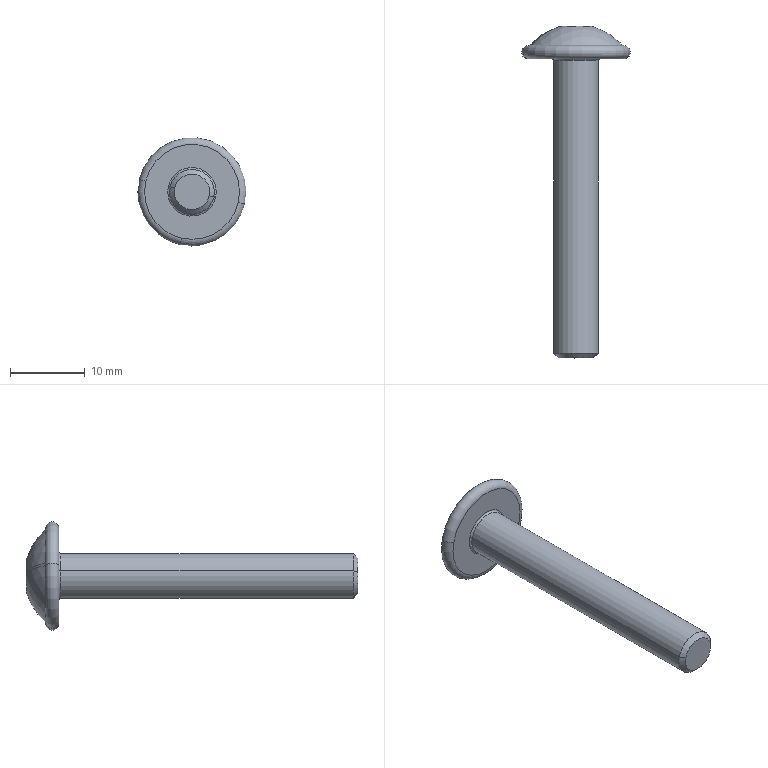Part | SolidWorks | features BaseBody 1 | 1 solid | 33 faces | box 14.5 x 44.401 x 14.5 mm | volume 1558 mm3 | cylinder 18 | torus 5 | sphere 4 | plane 4 | cone 2 | commonest cylinder face diameters 1.32 x6 3.14 x4 2.34 x3 6 x3 1.26 x2
STEP:
#1=CARTESIAN_POINT('',(2000.565,170.805,805.124));
#2=VERTEX_POINT('',#1);
#3=CARTESIAN_POINT('',(2002.818,170.805,801.529));
#4=VERTEX_POINT('',#3);
#5=CARTESIAN_POINT('',(2003.489,170.805,804.453));
#6=DIRECTION('',(0.,-1.,0.));
#7=DIRECTION('',(-0.9746,0.,0.2239));
#8=AXIS2_PLACEMENT_3D('',#5,#6,#7);
#9=CIRCLE('',#8,3.);
#10=EDGE_CURVE('',#2,#4,#9,.T.);
#11=ORIENTED_EDGE('',*,*,#10,.T.);
#12=CARTESIAN_POINT('',(2002.818,131.68,801.529));
#13=VERTEX_POINT('',#12);
#14=CARTESIAN_POINT('',(2002.818,171.588,801.529));
#15=DIRECTION('',(0.,-1.,0.));
#16=VECTOR('',#15,1000.);
#17=LINE('',#14,#16);
#18=EDGE_CURVE('',#4,#13,#17,.T.);
#19=ORIENTED_EDGE('',*,*,#18,.T.);
#20=CARTESIAN_POINT('',(2000.565,131.68,805.124));
#21=VERTEX_POINT('',#20);
#22=CARTESIAN_POINT('',(2003.489,131.68,804.453));
#23=DIRECTION('',(0.,-1.,0.));
#24=DIRECTION('',(-0.9746,0.,0.2239));
#25=AXIS2_PLACEMENT_3D('',#22,#23,#24);
#26=CIRCLE('',#25,3.);
#27=EDGE_CURVE('',#21,#13,#26,.T.);
#28=ORIENTED_EDGE('',*,*,#27,.F.);
#29=CARTESIAN_POINT('',(2000.565,170.805,805.124));
#30=DIRECTION('',(0.,-1.,0.));
#31=VECTOR('',#30,1000.);
#32=LINE('',#29,#31);
#33=EDGE_CURVE('',#2,#21,#32,.T.);
#34=ORIENTED_EDGE('',*,*,#33,.F.);
#35=EDGE_LOOP('',(#11,#19,#28,#34));
#36=FACE_OUTER_BOUND('',#35,.T.);
#37=CARTESIAN_POINT('',(2003.489,171.588,804.453));
#38=DIRECTION('',(0.,-1.,0.));
#39=DIRECTION('',(-0.2239,0.,-0.9746));
#40=AXIS2_PLACEMENT_3D('',#37,#38,#39);
#41=CYLINDRICAL_SURFACE('',#40,3.);
#42=ADVANCED_FACE('',(#36),#41,.T.);
#43=CARTESIAN_POINT('',(2003.924,175.456,806.344));
#44=VERTEX_POINT('',#43);
#45=CARTESIAN_POINT('',(2003.428,175.404,806.592));
#46=VERTEX_POINT('',#45);
#47=CARTESIAN_POINT('',(2003.924,175.456,806.344));
#48=CARTESIAN_POINT('',(2003.833,175.456,806.365));
#49=CARTESIAN_POINT('',(2003.743,175.451,806.397));
#50=CARTESIAN_POINT('',(2003.576,175.434,806.481));
#51=CARTESIAN_POINT('',(2003.499,175.421,806.532));
#52=CARTESIAN_POINT('',(2003.428,175.404,806.592));
#53=B_SPLINE_CURVE_WITH_KNOTS('',3,(#47,#48,#49,#50,#51,#52),.UNSPECIFIED.,.F.,.F.,(4,2,4),(0.0005602,0.0008404,0.001121),.UNSPECIFIED.);
#54=EDGE_CURVE('',#44,#46,#53,.T.);
#55=ORIENTED_EDGE('',*,*,#54,.F.);
#56=CARTESIAN_POINT('',(2003.924,173.205,806.344));
#57=VERTEX_POINT('',#56);
#58=CARTESIAN_POINT('',(2003.924,175.576,806.344));
#59=DIRECTION('',(0.,-1.,0.));
#60=VECTOR('',#59,1000.);
#61=LINE('',#58,#60);
#62=EDGE_CURVE('',#44,#57,#61,.T.);
#63=ORIENTED_EDGE('',*,*,#62,.T.);
#64=CARTESIAN_POINT('',(2003.428,173.205,806.592));
#65=VERTEX_POINT('',#64);
#66=CARTESIAN_POINT('',(2004.186,173.205,807.484));
#67=DIRECTION('',(0.,-1.,0.));
#68=DIRECTION('',(-0.6474,0.,-0.7622));
#69=AXIS2_PLACEMENT_3D('',#66,#67,#68);
#70=CIRCLE('',#69,1.17);
#71=EDGE_CURVE('',#65,#57,#70,.T.);
#72=ORIENTED_EDGE('',*,*,#71,.F.);
#73=CARTESIAN_POINT('',(2003.428,173.205,806.592));
#74=DIRECTION('',(0.,1.,0.));
#75=VECTOR('',#74,1000.);
#76=LINE('',#73,#75);
#77=EDGE_CURVE('',#65,#46,#76,.T.);
#78=ORIENTED_EDGE('',*,*,#77,.T.);
#79=EDGE_LOOP('',(#55,#63,#72,#78));
#80=FACE_OUTER_BOUND('',#79,.T.);
#81=CARTESIAN_POINT('',(2004.186,175.576,807.484));
#82=DIRECTION('',(0.,-1.,0.));
#83=DIRECTION('',(-0.2239,0.,-0.9746));
#84=AXIS2_PLACEMENT_3D('',#81,#82,#83);
#85=CYLINDRICAL_SURFACE('',#84,1.17);
#86=ADVANCED_FACE('',(#80),#85,.T.);
#87=CARTESIAN_POINT('',(2002.188,175.358,802.55));
#88=VERTEX_POINT('',#87);
#89=CARTESIAN_POINT('',(2002.501,175.404,802.555));
#90=VERTEX_POINT('',#89);
#91=CARTESIAN_POINT('',(2002.188,175.358,802.55));
#92=CARTESIAN_POINT('',(2002.291,175.369,802.527));
#93=CARTESIAN_POINT('',(2002.399,175.385,802.528));
#94=CARTESIAN_POINT('',(2002.501,175.404,802.555));
#95=B_SPLINE_CURVE_WITH_KNOTS('',3,(#91,#92,#93,#94),.UNSPECIFIED.,.F.,.F.,(4,4),(0.0009536,0.001271),.UNSPECIFIED.);
#96=EDGE_CURVE('',#88,#90,#95,.T.);
#97=ORIENTED_EDGE('',*,*,#96,.F.);
#98=CARTESIAN_POINT('',(2002.188,173.205,802.55));
#99=VERTEX_POINT('',#98);
#100=CARTESIAN_POINT('',(2002.188,175.524,802.55));
#101=DIRECTION('',(0.,-1.,0.));
#102=VECTOR('',#101,1000.);
#103=LINE('',#100,#102);
#104=EDGE_CURVE('',#88,#99,#103,.T.);
#105=ORIENTED_EDGE('',*,*,#104,.T.);
#106=CARTESIAN_POINT('',(2002.501,173.205,802.555));
#107=VERTEX_POINT('',#106);
#108=CARTESIAN_POINT('',(2002.336,173.205,803.194));
#109=DIRECTION('',(0.,1.,0.));
#110=DIRECTION('',(0.2499,0.,-0.9683));
#111=AXIS2_PLACEMENT_3D('',#108,#109,#110);
#112=CIRCLE('',#111,0.66);
#113=EDGE_CURVE('',#107,#99,#112,.T.);
#114=ORIENTED_EDGE('',*,*,#113,.F.);
#115=CARTESIAN_POINT('',(2002.501,173.205,802.555));
#116=DIRECTION('',(0.,1.,0.));
#117=VECTOR('',#116,1000.);
#118=LINE('',#115,#117);
#119=EDGE_CURVE('',#107,#90,#118,.T.);
#120=ORIENTED_EDGE('',*,*,#119,.T.);
#121=EDGE_LOOP('',(#97,#105,#114,#120));
#122=FACE_OUTER_BOUND('',#121,.T.);
#123=CARTESIAN_POINT('',(2002.336,175.524,803.194));
#124=DIRECTION('',(0.,-1.,0.));
#125=DIRECTION('',(-0.2239,0.,-0.9746));
#126=AXIS2_PLACEMENT_3D('',#123,#124,#125);
#127=CYLINDRICAL_SURFACE('',#126,0.66);
#128=ADVANCED_FACE('',(#122),#127,.F.);
#129=CARTESIAN_POINT('',(2003.83,175.358,802.173));
#130=VERTEX_POINT('',#129);
#131=CARTESIAN_POINT('',(2004.598,175.397,802.59));
#132=VERTEX_POINT('',#131);
#133=CARTESIAN_POINT('',(2003.83,175.358,802.173));
#134=CARTESIAN_POINT('',(2003.984,175.341,802.138));
#135=CARTESIAN_POINT('',(2004.154,175.335,802.161));
#136=CARTESIAN_POINT('',(2004.433,175.349,802.313));
#137=CARTESIAN_POINT('',(2004.543,175.369,802.441));
#138=CARTESIAN_POINT('',(2004.598,175.397,802.59));
#139=B_SPLINE_CURVE_WITH_KNOTS('',3,(#133,#134,#135,#136,#137,#138),.UNSPECIFIED.,.F.,.F.,(4,2,4),(0.0003176,0.0007942,0.001271),.UNSPECIFIED.);
#140=EDGE_CURVE('',#130,#132,#139,.T.);
#141=ORIENTED_EDGE('',*,*,#140,.F.);
#142=CARTESIAN_POINT('',(2003.83,173.205,802.173));
#143=VERTEX_POINT('',#142);
#144=CARTESIAN_POINT('',(2003.83,175.524,802.173));
#145=DIRECTION('',(0.,-1.,0.));
#146=VECTOR('',#145,1000.);
#147=LINE('',#144,#146);
#148=EDGE_CURVE('',#130,#143,#147,.T.);
#149=ORIENTED_EDGE('',*,*,#148,.T.);
#150=CARTESIAN_POINT('',(2004.598,173.205,802.59));
#151=VERTEX_POINT('',#150);
#152=CARTESIAN_POINT('',(2003.978,173.205,802.817));
#153=DIRECTION('',(0.,1.,0.));
#154=DIRECTION('',(0.9391,0.,-0.3438));
#155=AXIS2_PLACEMENT_3D('',#152,#153,#154);
#156=CIRCLE('',#155,0.66);
#157=EDGE_CURVE('',#151,#143,#156,.T.);
#158=ORIENTED_EDGE('',*,*,#157,.F.);
#159=CARTESIAN_POINT('',(2004.598,173.205,802.59));
#160=DIRECTION('',(0.,1.,0.));
#161=VECTOR('',#160,1000.);
#162=LINE('',#159,#161);
#163=EDGE_CURVE('',#151,#132,#162,.T.);
#164=ORIENTED_EDGE('',*,*,#163,.T.);
#165=EDGE_LOOP('',(#141,#149,#158,#164));
#166=FACE_OUTER_BOUND('',#165,.T.);
#167=CARTESIAN_POINT('',(2003.978,175.524,802.817));
#168=DIRECTION('',(0.,-1.,0.));
#169=DIRECTION('',(-0.2239,0.,-0.9746));
#170=AXIS2_PLACEMENT_3D('',#167,#168,#169);
#171=CYLINDRICAL_SURFACE('',#170,0.66);
#172=ADVANCED_FACE('',(#166),#171,.F.);
#173=CARTESIAN_POINT('',(2005.439,175.394,803.487));
#174=VERTEX_POINT('',#173);
#175=CARTESIAN_POINT('',(2005.749,175.342,803.782));
#176=VERTEX_POINT('',#175);
#177=CARTESIAN_POINT('',(2005.439,175.394,803.487));
#178=CARTESIAN_POINT('',(2005.572,175.369,803.546));
#179=CARTESIAN_POINT('',(2005.683,175.35,803.65));
#180=CARTESIAN_POINT('',(2005.749,175.342,803.782));
#181=B_SPLINE_CURVE_WITH_KNOTS('',3,(#177,#178,#179,#180),.UNSPECIFIED.,.F.,.F.,(4,4),(0.,0.0004379),.UNSPECIFIED.);
#182=EDGE_CURVE('',#174,#176,#181,.T.);
#183=ORIENTED_EDGE('',*,*,#182,.T.);
#184=CARTESIAN_POINT('',(2009.433,172.855,802.688));
#185=VERTEX_POINT('',#184);
#186=CARTESIAN_POINT('',(2003.489,167.488,804.453));
#187=DIRECTION('',(-0.2846,0.,-0.9586));
#188=DIRECTION('',(-0.9586,0.,0.2846));
#189=AXIS2_PLACEMENT_3D('',#186,#187,#188);
#190=CIRCLE('',#189,8.2);
#191=EDGE_CURVE('',#176,#185,#190,.T.);
#192=ORIENTED_EDGE('',*,*,#191,.T.);
#193=CARTESIAN_POINT('',(1997.447,172.855,805.841));
#194=VERTEX_POINT('',#193);
#195=CARTESIAN_POINT('',(2003.489,172.855,804.453));
#196=DIRECTION('',(0.,1.,0.));
#197=DIRECTION('',(0.9746,0.,-0.2239));
#198=AXIS2_PLACEMENT_3D('',#195,#196,#197);
#199=CIRCLE('',#198,6.2);
#200=EDGE_CURVE('',#185,#194,#199,.T.);
#201=ORIENTED_EDGE('',*,*,#200,.T.);
#202=CARTESIAN_POINT('',(2001.179,175.338,804.983));
#203=VERTEX_POINT('',#202);
#204=CARTESIAN_POINT('',(2003.489,167.488,804.453));
#205=DIRECTION('',(-0.2239,0.,-0.9746));
#206=DIRECTION('',(-0.7369,0.6545,0.1693));
#207=AXIS2_PLACEMENT_3D('',#204,#205,#206);
#208=CIRCLE('',#207,8.2);
#209=EDGE_CURVE('',#194,#203,#208,.T.);
#210=ORIENTED_EDGE('',*,*,#209,.T.);
#211=CARTESIAN_POINT('',(2001.313,175.394,804.434));
#212=VERTEX_POINT('',#211);
#213=CARTESIAN_POINT('',(2001.179,175.338,804.983));
#214=CARTESIAN_POINT('',(2001.135,175.338,804.79));
#215=CARTESIAN_POINT('',(2001.187,175.36,804.583));
#216=CARTESIAN_POINT('',(2001.313,175.394,804.434));
#217=B_SPLINE_CURVE_WITH_KNOTS('',3,(#213,#214,#215,#216),.UNSPECIFIED.,.F.,.F.,(4,4),(0.,0.000586),.UNSPECIFIED.);
#218=EDGE_CURVE('',#203,#212,#217,.T.);
#219=ORIENTED_EDGE('',*,*,#218,.T.);
#220=CARTESIAN_POINT('',(2001.679,175.397,803.26));
#221=VERTEX_POINT('',#220);
#222=CARTESIAN_POINT('',(2001.313,175.394,804.434));
#223=CARTESIAN_POINT('',(2001.381,175.413,804.354));
#224=CARTESIAN_POINT('',(2001.441,175.427,804.268));
#225=CARTESIAN_POINT('',(2001.542,175.446,804.085));
#226=CARTESIAN_POINT('',(2001.584,175.451,803.986));
#227=CARTESIAN_POINT('',(2001.679,175.452,803.684));
#228=CARTESIAN_POINT('',(2001.7,175.433,803.469));
#229=CARTESIAN_POINT('',(2001.679,175.397,803.26));
#230=B_SPLINE_CURVE_WITH_KNOTS('',3,(#222,#223,#224,#225,#226,#227,#228,#229),.UNSPECIFIED.,.F.,.F.,(4,2,2,4),(0.,0.0003157,0.0006314,0.001263),.UNSPECIFIED.);
#231=EDGE_CURVE('',#212,#221,#230,.T.);
#232=ORIENTED_EDGE('',*,*,#231,.T.);
#233=CARTESIAN_POINT('',(2001.679,175.397,803.26));
#234=CARTESIAN_POINT('',(2001.663,175.369,803.102));
#235=CARTESIAN_POINT('',(2001.706,175.35,802.94));
#236=CARTESIAN_POINT('',(2001.892,175.335,802.68));
#237=CARTESIAN_POINT('',(2002.034,175.341,802.586));
#238=CARTESIAN_POINT('',(2002.188,175.358,802.55));
#239=B_SPLINE_CURVE_WITH_KNOTS('',3,(#233,#234,#235,#236,#237,#238),.UNSPECIFIED.,.F.,.F.,(4,2,4),(0.,0.0004768,0.0009536),.UNSPECIFIED.);
#240=EDGE_CURVE('',#221,#88,#239,.T.);
#241=ORIENTED_EDGE('',*,*,#240,.T.);
#242=ORIENTED_EDGE('',*,*,#96,.T.);
#243=CARTESIAN_POINT('',(2003.55,175.404,802.314));
#244=VERTEX_POINT('',#243);
#245=CARTESIAN_POINT('',(2002.501,175.404,802.555));
#246=CARTESIAN_POINT('',(2002.591,175.421,802.578));
#247=CARTESIAN_POINT('',(2002.683,175.434,802.59));
#248=CARTESIAN_POINT('',(2002.869,175.451,802.593));
#249=CARTESIAN_POINT('',(2002.964,175.456,802.583));
#250=CARTESIAN_POINT('',(2003.146,175.456,802.541));
#251=CARTESIAN_POINT('',(2003.236,175.451,802.509));
#252=CARTESIAN_POINT('',(2003.402,175.434,802.425));
#253=CARTESIAN_POINT('',(2003.479,175.421,802.374));
#254=CARTESIAN_POINT('',(2003.55,175.404,802.314));
#255=B_SPLINE_CURVE_WITH_KNOTS('',3,(#245,#246,#247,#248,#249,#250,#251,#252,#253,#254),.UNSPECIFIED.,.F.,.F.,(4,2,2,2,4),(0.,0.0002801,0.0005603,0.0008404,0.001121),.UNSPECIFIED.);
#256=EDGE_CURVE('',#90,#244,#255,.T.);
#257=ORIENTED_EDGE('',*,*,#256,.T.);
#258=CARTESIAN_POINT('',(2003.55,175.404,802.314));
#259=CARTESIAN_POINT('',(2003.631,175.385,802.245));
#260=CARTESIAN_POINT('',(2003.727,175.369,802.197));
#261=CARTESIAN_POINT('',(2003.83,175.358,802.173));
#262=B_SPLINE_CURVE_WITH_KNOTS('',3,(#258,#259,#260,#261),.UNSPECIFIED.,.F.,.F.,(4,4),(0.,0.0003176),.UNSPECIFIED.);
#263=EDGE_CURVE('',#244,#130,#262,.T.);
#264=ORIENTED_EDGE('',*,*,#263,.T.);
#265=ORIENTED_EDGE('',*,*,#140,.T.);
#266=CARTESIAN_POINT('',(2004.598,175.397,802.59));
#267=CARTESIAN_POINT('',(2004.634,175.415,802.688));
#268=CARTESIAN_POINT('',(2004.679,175.429,802.782));
#269=CARTESIAN_POINT('',(2004.789,175.447,802.961));
#270=CARTESIAN_POINT('',(2004.854,175.452,803.047));
#271=CARTESIAN_POINT('',(2005.071,175.451,803.278));
#272=CARTESIAN_POINT('',(2005.247,175.432,803.402));
#273=CARTESIAN_POINT('',(2005.439,175.394,803.487));
#274=B_SPLINE_CURVE_WITH_KNOTS('',3,(#266,#267,#268,#269,#270,#271,#272,#273),.UNSPECIFIED.,.F.,.F.,(4,2,2,4),(0.,0.0003157,0.0006314,0.001263),.UNSPECIFIED.);
#275=EDGE_CURVE('',#132,#174,#274,.T.);
#276=ORIENTED_EDGE('',*,*,#275,.T.);
#277=EDGE_LOOP('',(#183,#192,#201,#210,#219,#232,#241,#242,#257,#264,#265,#276));
#278=FACE_OUTER_BOUND('',#277,.T.);
#279=CARTESIAN_POINT('',(2003.489,167.488,804.453));
#280=DIRECTION('',(-0.2846,0.,-0.9586));
#281=DIRECTION('',(-0.9586,0.,0.2846));
#282=AXIS2_PLACEMENT_3D('',#279,#280,#281);
#283=SPHERICAL_SURFACE('',#282,8.2);
#284=ADVANCED_FACE('',(#278),#283,.T.);
#285=CARTESIAN_POINT('',(2001.54,175.394,805.419));
#286=VERTEX_POINT('',#285);
#287=CARTESIAN_POINT('',(2001.23,175.342,805.124));
#288=VERTEX_POINT('',#287);
#289=CARTESIAN_POINT('',(2001.54,175.394,805.419));
#290=CARTESIAN_POINT('',(2001.406,175.369,805.36));
#291=CARTESIAN_POINT('',(2001.296,175.35,805.256));
#292=CARTESIAN_POINT('',(2001.23,175.342,805.124));
#293=B_SPLINE_CURVE_WITH_KNOTS('',3,(#289,#290,#291,#292),.UNSPECIFIED.,.F.,.F.,(4,4),(0.,0.0004379),.UNSPECIFIED.);
#294=EDGE_CURVE('',#286,#288,#293,.T.);
#295=ORIENTED_EDGE('',*,*,#294,.T.);
#296=CARTESIAN_POINT('',(1997.546,172.855,806.218));
#297=VERTEX_POINT('',#296);
#298=CARTESIAN_POINT('',(2003.489,167.488,804.453));
#299=DIRECTION('',(0.2846,0.,0.9586));
#300=DIRECTION('',(0.9586,0.,-0.2846));
#301=AXIS2_PLACEMENT_3D('',#298,#299,#300);
#302=CIRCLE('',#301,8.2);
#303=EDGE_CURVE('',#288,#297,#302,.T.);
#304=ORIENTED_EDGE('',*,*,#303,.T.);
#305=CARTESIAN_POINT('',(2009.532,172.855,803.065));
#306=VERTEX_POINT('',#305);
#307=CARTESIAN_POINT('',(2003.489,172.855,804.453));
#308=DIRECTION('',(0.,-1.,0.));
#309=DIRECTION('',(0.9746,0.,-0.2239));
#310=AXIS2_PLACEMENT_3D('',#307,#308,#309);
#311=CIRCLE('',#310,6.2);
#312=EDGE_CURVE('',#306,#297,#311,.T.);
#313=ORIENTED_EDGE('',*,*,#312,.F.);
#314=CARTESIAN_POINT('',(2005.799,175.338,803.922));
#315=VERTEX_POINT('',#314);
#316=CARTESIAN_POINT('',(2003.489,167.488,804.453));
#317=DIRECTION('',(-0.2239,0.,-0.9746));
#318=DIRECTION('',(0.7369,0.6545,-0.1693));
#319=AXIS2_PLACEMENT_3D('',#316,#317,#318);
#320=CIRCLE('',#319,8.2);
#321=EDGE_CURVE('',#315,#306,#320,.T.);
#322=ORIENTED_EDGE('',*,*,#321,.F.);
#323=CARTESIAN_POINT('',(2005.665,175.394,804.471));
#324=VERTEX_POINT('',#323);
#325=CARTESIAN_POINT('',(2005.799,175.338,803.922));
#326=CARTESIAN_POINT('',(2005.843,175.338,804.115));
#327=CARTESIAN_POINT('',(2005.792,175.36,804.323));
#328=CARTESIAN_POINT('',(2005.665,175.394,804.471));
#329=B_SPLINE_CURVE_WITH_KNOTS('',3,(#325,#326,#327,#328),.UNSPECIFIED.,.F.,.F.,(4,4),(0.,0.000586),.UNSPECIFIED.);
#330=EDGE_CURVE('',#315,#324,#329,.T.);
#331=ORIENTED_EDGE('',*,*,#330,.T.);
#332=CARTESIAN_POINT('',(2005.299,175.397,805.646));
#333=VERTEX_POINT('',#332);
#334=CARTESIAN_POINT('',(2005.665,175.394,804.471));
#335=CARTESIAN_POINT('',(2005.597,175.413,804.551));
#336=CARTESIAN_POINT('',(2005.538,175.427,804.637));
#337=CARTESIAN_POINT('',(2005.436,175.446,804.821));
#338=CARTESIAN_POINT('',(2005.394,175.451,804.92));
#339=CARTESIAN_POINT('',(2005.3,175.452,805.222));
#340=CARTESIAN_POINT('',(2005.278,175.433,805.436));
#341=CARTESIAN_POINT('',(2005.299,175.397,805.646));
#342=B_SPLINE_CURVE_WITH_KNOTS('',3,(#334,#335,#336,#337,#338,#339,#340,#341),.UNSPECIFIED.,.F.,.F.,(4,2,2,4),(0.,0.0003157,0.0006314,0.001263),.UNSPECIFIED.);
#343=EDGE_CURVE('',#324,#333,#342,.T.);
#344=ORIENTED_EDGE('',*,*,#343,.T.);
#345=CARTESIAN_POINT('',(2004.478,175.404,806.351));
#346=VERTEX_POINT('',#345);
#347=CARTESIAN_POINT('',(2005.299,175.397,805.646));
#348=CARTESIAN_POINT('',(2005.31,175.378,805.751));
#349=CARTESIAN_POINT('',(2005.295,175.363,805.858));
#350=CARTESIAN_POINT('',(2005.217,175.344,806.054));
#351=CARTESIAN_POINT('',(2005.154,175.339,806.143));
#352=CARTESIAN_POINT('',(2004.992,175.34,806.282));
#353=CARTESIAN_POINT('',(2004.894,175.347,806.331));
#354=CARTESIAN_POINT('',(2004.688,175.369,806.379));
#355=CARTESIAN_POINT('',(2004.58,175.385,806.377));
#356=CARTESIAN_POINT('',(2004.478,175.404,806.351));
#357=B_SPLINE_CURVE_WITH_KNOTS('',3,(#347,#348,#349,#350,#351,#352,#353,#354,#355,#356),.UNSPECIFIED.,.F.,.F.,(4,2,2,2,4),(0.,0.0003177,0.0006354,0.0009531,0.001271),.UNSPECIFIED.);
#358=EDGE_CURVE('',#333,#346,#357,.T.);
#359=ORIENTED_EDGE('',*,*,#358,.T.);
#360=CARTESIAN_POINT('',(2004.478,175.404,806.351));
#361=CARTESIAN_POINT('',(2004.388,175.421,806.328));
#362=CARTESIAN_POINT('',(2004.296,175.434,806.315));
#363=CARTESIAN_POINT('',(2004.109,175.451,806.313));
#364=CARTESIAN_POINT('',(2004.015,175.456,806.323));
#365=CARTESIAN_POINT('',(2003.924,175.456,806.344));
#366=B_SPLINE_CURVE_WITH_KNOTS('',3,(#360,#361,#362,#363,#364,#365),.UNSPECIFIED.,.F.,.F.,(4,2,4),(0.,0.0002801,0.0005602),.UNSPECIFIED.);
#367=EDGE_CURVE('',#346,#44,#366,.T.);
#368=ORIENTED_EDGE('',*,*,#367,.T.);
#369=ORIENTED_EDGE('',*,*,#54,.T.);
#370=CARTESIAN_POINT('',(2002.381,175.397,806.316));
#371=VERTEX_POINT('',#370);
#372=CARTESIAN_POINT('',(2003.428,175.404,806.592));
#373=CARTESIAN_POINT('',(2003.348,175.385,806.661));
#374=CARTESIAN_POINT('',(2003.251,175.369,806.709));
#375=CARTESIAN_POINT('',(2003.046,175.347,806.756));
#376=CARTESIAN_POINT('',(2002.937,175.34,806.755));
#377=CARTESIAN_POINT('',(2002.73,175.338,806.701));
#378=CARTESIAN_POINT('',(2002.634,175.343,806.648));
#379=CARTESIAN_POINT('',(2002.478,175.363,806.505));
#380=CARTESIAN_POINT('',(2002.417,175.378,806.415));
#381=CARTESIAN_POINT('',(2002.381,175.397,806.316));
#382=B_SPLINE_CURVE_WITH_KNOTS('',3,(#372,#373,#374,#375,#376,#377,#378,#379,#380,#381),.UNSPECIFIED.,.F.,.F.,(4,2,2,2,4),(0.,0.0003177,0.0006354,0.000953,0.001271),.UNSPECIFIED.);
#383=EDGE_CURVE('',#46,#371,#382,.T.);
#384=ORIENTED_EDGE('',*,*,#383,.T.);
#385=CARTESIAN_POINT('',(2002.381,175.397,806.316));
#386=CARTESIAN_POINT('',(2002.345,175.415,806.217));
#387=CARTESIAN_POINT('',(2002.299,175.429,806.123));
#388=CARTESIAN_POINT('',(2002.189,175.447,805.944));
#389=CARTESIAN_POINT('',(2002.124,175.452,805.859));
#390=CARTESIAN_POINT('',(2001.908,175.451,805.628));
#391=CARTESIAN_POINT('',(2001.732,175.432,805.504));
#392=CARTESIAN_POINT('',(2001.54,175.394,805.419));
#393=B_SPLINE_CURVE_WITH_KNOTS('',3,(#385,#386,#387,#388,#389,#390,#391,#392),.UNSPECIFIED.,.F.,.F.,(4,2,2,4),(0.,0.0003157,0.0006314,0.001263),.UNSPECIFIED.);
#394=EDGE_CURVE('',#371,#286,#393,.T.);
#395=ORIENTED_EDGE('',*,*,#394,.T.);
#396=EDGE_LOOP('',(#295,#304,#313,#322,#331,#344,#359,#368,#369,#384,#395));
#397=FACE_OUTER_BOUND('',#396,.T.);
#398=CARTESIAN_POINT('',(2003.489,167.488,804.453));
#399=DIRECTION('',(0.2846,0.,0.9586));
#400=DIRECTION('',(0.9586,0.,-0.2846));
#401=AXIS2_PLACEMENT_3D('',#398,#399,#400);
#402=SPHERICAL_SURFACE('',#401,8.2);
#403=ADVANCED_FACE('',(#397),#402,.T.);
#404=CARTESIAN_POINT('',(2002.068,172.855,798.264));
#405=VERTEX_POINT('',#404);
#406=CARTESIAN_POINT('',(1997.3,172.855,805.874));
#407=VERTEX_POINT('',#406);
#408=CARTESIAN_POINT('',(2003.489,172.855,804.453));
#409=DIRECTION('',(0.,1.,0.));
#410=DIRECTION('',(0.9746,0.,-0.2239));
#411=AXIS2_PLACEMENT_3D('',#408,#409,#410);
#412=CIRCLE('',#411,6.35);
#413=EDGE_CURVE('',#405,#407,#412,.T.);
#414=ORIENTED_EDGE('',*,*,#413,.F.);
#415=CARTESIAN_POINT('',(2002.068,171.055,798.264));
#416=VERTEX_POINT('',#415);
#417=CARTESIAN_POINT('',(2002.068,171.955,798.264));
#418=DIRECTION('',(-0.9746,0.,0.2239));
#419=DIRECTION('',(0.2239,0.,0.9746));
#420=AXIS2_PLACEMENT_3D('',#417,#418,#419);
#421=CIRCLE('',#420,0.9);
#422=EDGE_CURVE('',#405,#416,#421,.T.);
#423=ORIENTED_EDGE('',*,*,#422,.T.);
#424=CARTESIAN_POINT('',(1997.3,171.055,805.874));
#425=VERTEX_POINT('',#424);
#426=CARTESIAN_POINT('',(2003.489,171.055,804.453));
#427=DIRECTION('',(0.,1.,0.));
#428=DIRECTION('',(0.9746,0.,-0.2239));
#429=AXIS2_PLACEMENT_3D('',#426,#427,#428);
#430=CIRCLE('',#429,6.35);
#431=EDGE_CURVE('',#416,#425,#430,.T.);
#432=ORIENTED_EDGE('',*,*,#431,.T.);
#433=CARTESIAN_POINT('',(1997.3,171.955,805.874));
#434=DIRECTION('',(0.2239,0.,0.9746));
#435=DIRECTION('',(0.,-1.,0.));
#436=AXIS2_PLACEMENT_3D('',#433,#434,#435);
#437=CIRCLE('',#436,0.9);
#438=EDGE_CURVE('',#407,#425,#437,.T.);
#439=ORIENTED_EDGE('',*,*,#438,.F.);
#440=EDGE_LOOP('',(#414,#423,#432,#439));
#441=FACE_OUTER_BOUND('',#440,.T.);
#442=CARTESIAN_POINT('',(2003.489,171.955,804.453));
#443=DIRECTION('',(0.,-1.,0.));
#444=DIRECTION('',(-0.2239,0.,-0.9746));
#445=AXIS2_PLACEMENT_3D('',#442,#443,#444);
#446=TOROIDAL_SURFACE('',#445,6.35,0.9);
#447=ADVANCED_FACE('',(#441),#446,.T.);
#448=CARTESIAN_POINT('',(2005.804,131.055,803.921));
#449=VERTEX_POINT('',#448);
#450=CARTESIAN_POINT('',(2001.175,131.055,804.985));
#451=VERTEX_POINT('',#450);
#452=CARTESIAN_POINT('',(2003.489,131.055,804.453));
#453=DIRECTION('',(0.,-1.,0.));
#454=DIRECTION('',(0.9746,0.,-0.2239));
#455=AXIS2_PLACEMENT_3D('',#452,#453,#454);
#456=CIRCLE('',#455,2.375);
#457=EDGE_CURVE('',#449,#451,#456,.T.);
#458=ORIENTED_EDGE('',*,*,#457,.T.);
#459=CARTESIAN_POINT('',(2003.489,131.055,804.453));
#460=DIRECTION('',(0.,-1.,0.));
#461=DIRECTION('',(-0.9746,0.,0.2239));
#462=AXIS2_PLACEMENT_3D('',#459,#460,#461);
#463=CIRCLE('',#462,2.375);
#464=EDGE_CURVE('',#451,#449,#463,.T.);
#465=ORIENTED_EDGE('',*,*,#464,.T.);
#466=EDGE_LOOP('',(#458,#465));
#467=FACE_OUTER_BOUND('',#466,.T.);
#468=CARTESIAN_POINT('',(2006.48,131.055,806.326));
#469=DIRECTION('',(0.,-1.,0.));
#470=DIRECTION('',(-0.9746,0.,0.2239));
#471=AXIS2_PLACEMENT_3D('',#468,#469,#470);
#472=PLANE('',#471);
#473=ADVANCED_FACE('',(#467),#472,.T.);
#474=CARTESIAN_POINT('',(2001.175,131.055,804.985));
#475=DIRECTION('',(-0.6892,0.7071,0.1583));
#476=VECTOR('',#475,1000.);
#477=LINE('',#474,#476);
#478=EDGE_CURVE('',#451,#21,#477,.T.);
#479=ORIENTED_EDGE('',*,*,#478,.T.);
#480=ORIENTED_EDGE('',*,*,#27,.T.);
#481=CARTESIAN_POINT('',(2006.413,131.68,803.781));
#482=VERTEX_POINT('',#481);
#483=CARTESIAN_POINT('',(2003.489,131.68,804.453));
#484=DIRECTION('',(0.,-1.,0.));
#485=DIRECTION('',(-0.9746,0.,0.2239));
#486=AXIS2_PLACEMENT_3D('',#483,#484,#485);
#487=CIRCLE('',#486,3.);
#488=EDGE_CURVE('',#13,#482,#487,.T.);
#489=ORIENTED_EDGE('',*,*,#488,.T.);
#490=CARTESIAN_POINT('',(2005.804,131.055,803.921));
#491=DIRECTION('',(-0.6892,-0.7071,0.1583));
#492=VECTOR('',#491,1000.);
#493=LINE('',#490,#492);
#494=EDGE_CURVE('',#482,#449,#493,.T.);
#495=ORIENTED_EDGE('',*,*,#494,.T.);
#496=ORIENTED_EDGE('',*,*,#464,.F.);
#497=EDGE_LOOP('',(#479,#480,#489,#495,#496));
#498=FACE_OUTER_BOUND('',#497,.T.);
#499=CARTESIAN_POINT('',(2003.489,131.765,804.453));
#500=DIRECTION('',(0.,1.,0.));
#501=DIRECTION('',(-0.9746,0.,0.2239));
#502=AXIS2_PLACEMENT_3D('',#499,#500,#501);
#503=CONICAL_SURFACE('',#502,3.085,0.7854);
#504=ADVANCED_FACE('',(#498),#503,.T.);
#505=ORIENTED_EDGE('',*,*,#494,.F.);
#506=CARTESIAN_POINT('',(2003.489,131.68,804.453));
#507=DIRECTION('',(0.,-1.,0.));
#508=DIRECTION('',(0.9746,0.,-0.2239));
#509=AXIS2_PLACEMENT_3D('',#506,#507,#508);
#510=CIRCLE('',#509,3.);
#511=EDGE_CURVE('',#482,#21,#510,.T.);
#512=ORIENTED_EDGE('',*,*,#511,.T.);
#513=ORIENTED_EDGE('',*,*,#478,.F.);
#514=ORIENTED_EDGE('',*,*,#457,.F.);
#515=EDGE_LOOP('',(#505,#512,#513,#514));
#516=FACE_OUTER_BOUND('',#515,.T.);
#517=CARTESIAN_POINT('',(2003.489,131.765,804.453));
#518=DIRECTION('',(0.,1.,0.));
#519=DIRECTION('',(-0.9746,0.,0.2239));
#520=AXIS2_PLACEMENT_3D('',#517,#518,#519);
#521=CONICAL_SURFACE('',#520,3.085,0.7854);
#522=ADVANCED_FACE('',(#516),#521,.T.);
#523=ORIENTED_EDGE('',*,*,#33,.T.);
#524=ORIENTED_EDGE('',*,*,#511,.F.);
#525=CARTESIAN_POINT('',(2006.413,170.805,803.781));
#526=VERTEX_POINT('',#525);
#527=CARTESIAN_POINT('',(2006.413,170.805,803.781));
#528=DIRECTION('',(0.,1.,0.));
#529=VECTOR('',#528,1000.);
#530=LINE('',#527,#529);
#531=EDGE_CURVE('',#482,#526,#530,.T.);
#532=ORIENTED_EDGE('',*,*,#531,.T.);
#533=CARTESIAN_POINT('',(2003.489,170.805,804.453));
#534=DIRECTION('',(0.,-1.,0.));
#535=DIRECTION('',(0.9746,0.,-0.2239));
#536=AXIS2_PLACEMENT_3D('',#533,#534,#535);
#537=CIRCLE('',#536,3.);
#538=EDGE_CURVE('',#526,#2,#537,.T.);
#539=ORIENTED_EDGE('',*,*,#538,.T.);
#540=EDGE_LOOP('',(#523,#524,#532,#539));
#541=FACE_OUTER_BOUND('',#540,.T.);
#542=CARTESIAN_POINT('',(2003.489,171.588,804.453));
#543=DIRECTION('',(0.,-1.,0.));
#544=DIRECTION('',(-0.2239,0.,-0.9746));
#545=AXIS2_PLACEMENT_3D('',#542,#543,#544);
#546=CYLINDRICAL_SURFACE('',#545,3.);
#547=ADVANCED_FACE('',(#541),#546,.T.);
#548=CARTESIAN_POINT('',(2000.322,171.055,805.18));
#549=VERTEX_POINT('',#548);
#550=CARTESIAN_POINT('',(2000.322,170.805,805.18));
#551=DIRECTION('',(-0.2239,0.,-0.9746));
#552=DIRECTION('',(0.000000004,1.,-0.000000001));
#553=AXIS2_PLACEMENT_3D('',#550,#551,#552);
#554=CIRCLE('',#553,0.25);
#555=EDGE_CURVE('',#549,#2,#554,.T.);
#556=ORIENTED_EDGE('',*,*,#555,.T.);
#557=ORIENTED_EDGE('',*,*,#538,.F.);
#558=CARTESIAN_POINT('',(2006.657,171.055,803.725));
#559=VERTEX_POINT('',#558);
#560=CARTESIAN_POINT('',(2006.657,170.805,803.725));
#561=DIRECTION('',(-0.2239,0.,-0.9746));
#562=DIRECTION('',(-0.000000004,1.,0.000000001));
#563=AXIS2_PLACEMENT_3D('',#560,#561,#562);
#564=CIRCLE('',#563,0.25);
#565=EDGE_CURVE('',#526,#559,#564,.T.);
#566=ORIENTED_EDGE('',*,*,#565,.T.);
#567=CARTESIAN_POINT('',(2003.489,171.055,804.453));
#568=DIRECTION('',(0.,-1.,0.));
#569=DIRECTION('',(0.9746,0.,-0.2239));
#570=AXIS2_PLACEMENT_3D('',#567,#568,#569);
#571=CIRCLE('',#570,3.25);
#572=EDGE_CURVE('',#559,#549,#571,.T.);
#573=ORIENTED_EDGE('',*,*,#572,.T.);
#574=EDGE_LOOP('',(#556,#557,#566,#573));
#575=FACE_OUTER_BOUND('',#574,.T.);
#576=CARTESIAN_POINT('',(2003.489,170.805,804.453));
#577=DIRECTION('',(0.,-1.,0.));
#578=DIRECTION('',(0.9746,0.,-0.2239));
#579=AXIS2_PLACEMENT_3D('',#576,#577,#578);
#580=TOROIDAL_SURFACE('',#579,3.25,0.25);
#581=ADVANCED_FACE('',(#575),#580,.F.);
#582=CARTESIAN_POINT('',(2009.678,171.055,803.031));
#583=VERTEX_POINT('',#582);
#584=CARTESIAN_POINT('',(2003.489,171.055,804.453));
#585=DIRECTION('',(0.,1.,0.));
#586=DIRECTION('',(0.9746,0.,-0.2239));
#587=AXIS2_PLACEMENT_3D('',#584,#585,#586);
#588=CIRCLE('',#587,6.35);
#589=EDGE_CURVE('',#583,#416,#588,.T.);
#590=ORIENTED_EDGE('',*,*,#589,.F.);
#591=CARTESIAN_POINT('',(2003.489,171.055,804.453));
#592=DIRECTION('',(0.,-1.,0.));
#593=DIRECTION('',(0.9746,0.,-0.2239));
#594=AXIS2_PLACEMENT_3D('',#591,#592,#593);
#595=CIRCLE('',#594,6.35);
#596=EDGE_CURVE('',#583,#425,#595,.T.);
#597=ORIENTED_EDGE('',*,*,#596,.T.);
#598=ORIENTED_EDGE('',*,*,#431,.F.);
#599=EDGE_LOOP('',(#590,#597,#598));
#600=FACE_OUTER_BOUND('',#599,.T.);
#601=ORIENTED_EDGE('',*,*,#572,.F.);
#602=CARTESIAN_POINT('',(2003.489,171.055,804.453));
#603=DIRECTION('',(0.,-1.,0.));
#604=DIRECTION('',(-0.9746,0.,0.2239));
#605=AXIS2_PLACEMENT_3D('',#602,#603,#604);
#606=CIRCLE('',#605,3.25);
#607=EDGE_CURVE('',#549,#559,#606,.T.);
#608=ORIENTED_EDGE('',*,*,#607,.F.);
#609=EDGE_LOOP('',(#601,#608));
#610=FACE_BOUND('',#609,.T.);
#611=CARTESIAN_POINT('',(2011.408,171.055,809.429));
#612=DIRECTION('',(0.,-1.,0.));
#613=DIRECTION('',(-0.9746,0.,0.2239));
#614=AXIS2_PLACEMENT_3D('',#611,#612,#613);
#615=PLANE('',#614);
#616=ADVANCED_FACE('',(#600,#610),#615,.T.);
#617=CARTESIAN_POINT('',(2009.678,172.855,803.031));
#618=VERTEX_POINT('',#617);
#619=CARTESIAN_POINT('',(2003.489,172.855,804.453));
#620=DIRECTION('',(0.,-1.,0.));
#621=DIRECTION('',(0.9746,0.,-0.2239));
#622=AXIS2_PLACEMENT_3D('',#619,#620,#621);
#623=CIRCLE('',#622,6.35);
#624=EDGE_CURVE('',#618,#407,#623,.T.);
#625=ORIENTED_EDGE('',*,*,#624,.T.);
#626=ORIENTED_EDGE('',*,*,#438,.T.);
#627=ORIENTED_EDGE('',*,*,#596,.F.);
#628=CARTESIAN_POINT('',(2009.678,171.955,803.031));
#629=DIRECTION('',(0.2239,0.,0.9746));
#630=DIRECTION('',(0.,-1.,0.));
#631=AXIS2_PLACEMENT_3D('',#628,#629,#630);
#632=CIRCLE('',#631,0.9);
#633=EDGE_CURVE('',#583,#618,#632,.T.);
#634=ORIENTED_EDGE('',*,*,#633,.T.);
#635=EDGE_LOOP('',(#625,#626,#627,#634));
#636=FACE_OUTER_BOUND('',#635,.T.);
#637=CARTESIAN_POINT('',(2003.489,171.955,804.453));
#638=DIRECTION('',(0.,-1.,0.));
#639=DIRECTION('',(-0.2239,0.,-0.9746));
#640=AXIS2_PLACEMENT_3D('',#637,#638,#639);
#641=TOROIDAL_SURFACE('',#640,6.35,0.9);
#642=ADVANCED_FACE('',(#636),#641,.T.);
#643=ORIENTED_EDGE('',*,*,#422,.F.);
#644=CARTESIAN_POINT('',(2003.489,172.855,804.453));
#645=DIRECTION('',(0.,1.,0.));
#646=DIRECTION('',(0.9746,0.,-0.2239));
#647=AXIS2_PLACEMENT_3D('',#644,#645,#646);
#648=CIRCLE('',#647,6.35);
#649=EDGE_CURVE('',#618,#405,#648,.T.);
#650=ORIENTED_EDGE('',*,*,#649,.F.);
#651=ORIENTED_EDGE('',*,*,#633,.F.);
#652=ORIENTED_EDGE('',*,*,#589,.T.);
#653=EDGE_LOOP('',(#643,#650,#651,#652));
#654=FACE_OUTER_BOUND('',#653,.T.);
#655=CARTESIAN_POINT('',(2003.489,171.955,804.453));
#656=DIRECTION('',(0.,-1.,0.));
#657=DIRECTION('',(-0.2239,0.,-0.9746));
#658=AXIS2_PLACEMENT_3D('',#655,#656,#657);
#659=TOROIDAL_SURFACE('',#658,6.35,0.9);
#660=ADVANCED_FACE('',(#654),#659,.T.);
#661=ORIENTED_EDGE('',*,*,#624,.F.);
#662=ORIENTED_EDGE('',*,*,#649,.T.);
#663=ORIENTED_EDGE('',*,*,#413,.T.);
#664=EDGE_LOOP('',(#661,#662,#663));
#665=FACE_OUTER_BOUND('',#664,.T.);
#666=CARTESIAN_POINT('',(2003.489,172.855,804.453));
#667=DIRECTION('',(0.,1.,0.));
#668=DIRECTION('',(0.9746,0.,-0.2239));
#669=AXIS2_PLACEMENT_3D('',#666,#667,#668);
#670=CIRCLE('',#669,6.2);
#671=EDGE_CURVE('',#306,#185,#670,.T.);
#672=ORIENTED_EDGE('',*,*,#671,.F.);
#673=ORIENTED_EDGE('',*,*,#312,.T.);
#674=CARTESIAN_POINT('',(2003.489,172.855,804.453));
#675=DIRECTION('',(0.,-1.,0.));
#676=DIRECTION('',(0.9746,0.,-0.2239));
#677=AXIS2_PLACEMENT_3D('',#674,#675,#676);
#678=CIRCLE('',#677,6.2);
#679=EDGE_CURVE('',#297,#194,#678,.T.);
#680=ORIENTED_EDGE('',*,*,#679,.T.);
#681=ORIENTED_EDGE('',*,*,#200,.F.);
#682=EDGE_LOOP('',(#672,#673,#680,#681));
#683=FACE_BOUND('',#682,.T.);
#684=CARTESIAN_POINT('',(2011.408,172.855,809.429));
#685=DIRECTION('',(0.,1.,0.));
#686=DIRECTION('',(-0.2239,0.,-0.9746));
#687=AXIS2_PLACEMENT_3D('',#684,#685,#686);
#688=PLANE('',#687);
#689=ADVANCED_FACE('',(#665,#683),#688,.T.);
#690=ORIENTED_EDGE('',*,*,#303,.F.);
#691=CARTESIAN_POINT('',(2001.23,175.342,805.124));
#692=CARTESIAN_POINT('',(2001.207,175.34,805.079));
#693=CARTESIAN_POINT('',(2001.191,175.338,805.032));
#694=CARTESIAN_POINT('',(2001.179,175.338,804.983));
#695=B_SPLINE_CURVE_WITH_KNOTS('',3,(#691,#692,#693,#694),.UNSPECIFIED.,.F.,.F.,(4,4),(0.0004379,0.0005861),.UNSPECIFIED.);
#696=EDGE_CURVE('',#288,#203,#695,.T.);
#697=ORIENTED_EDGE('',*,*,#696,.T.);
#698=ORIENTED_EDGE('',*,*,#209,.F.);
#699=ORIENTED_EDGE('',*,*,#679,.F.);
#700=EDGE_LOOP('',(#690,#697,#698,#699));
#701=FACE_OUTER_BOUND('',#700,.T.);
#702=CARTESIAN_POINT('',(2003.489,167.488,804.453));
#703=DIRECTION('',(0.2846,0.,0.9586));
#704=DIRECTION('',(0.9586,0.,-0.2846));
#705=AXIS2_PLACEMENT_3D('',#702,#703,#704);
#706=SPHERICAL_SURFACE('',#705,8.2);
#707=ADVANCED_FACE('',(#701),#706,.T.);
#708=CARTESIAN_POINT('',(2001.313,173.205,804.434));
#709=VERTEX_POINT('',#708);
#710=CARTESIAN_POINT('',(2001.54,173.205,805.419));
#711=VERTEX_POINT('',#710);
#712=CARTESIAN_POINT('',(2001.793,173.205,804.842));
#713=DIRECTION('',(0.,1.,0.));
#714=DIRECTION('',(-0.762,0.,-0.6476));
#715=AXIS2_PLACEMENT_3D('',#712,#713,#714);
#716=CIRCLE('',#715,0.63);
#717=EDGE_CURVE('',#709,#711,#716,.T.);
#718=ORIENTED_EDGE('',*,*,#717,.F.);
#719=CARTESIAN_POINT('',(2001.313,173.205,804.434));
#720=DIRECTION('',(0.,1.,0.));
#721=VECTOR('',#720,1000.);
#722=LINE('',#719,#721);
#723=EDGE_CURVE('',#709,#212,#722,.T.);
#724=ORIENTED_EDGE('',*,*,#723,.T.);
#725=ORIENTED_EDGE('',*,*,#218,.F.);
#726=ORIENTED_EDGE('',*,*,#696,.F.);
#727=ORIENTED_EDGE('',*,*,#294,.F.);
#728=CARTESIAN_POINT('',(2001.54,173.205,805.419));
#729=DIRECTION('',(0.,1.,0.));
#730=VECTOR('',#729,1000.);
#731=LINE('',#728,#730);
#732=EDGE_CURVE('',#711,#286,#731,.T.);
#733=ORIENTED_EDGE('',*,*,#732,.F.);
#734=EDGE_LOOP('',(#718,#724,#725,#726,#727,#733));
#735=FACE_OUTER_BOUND('',#734,.T.);
#736=CARTESIAN_POINT('',(2001.793,175.514,804.842));
#737=DIRECTION('',(0.,-1.,0.));
#738=DIRECTION('',(-0.2239,0.,-0.9746));
#739=AXIS2_PLACEMENT_3D('',#736,#737,#738);
#740=CYLINDRICAL_SURFACE('',#739,0.63);
#741=ADVANCED_FACE('',(#735),#740,.F.);
#742=ORIENTED_EDGE('',*,*,#394,.F.);
#743=CARTESIAN_POINT('',(2002.381,173.205,806.316));
#744=VERTEX_POINT('',#743);
#745=CARTESIAN_POINT('',(2002.381,173.205,806.316));
#746=DIRECTION('',(0.,1.,0.));
#747=VECTOR('',#746,1000.);
#748=LINE('',#745,#747);
#749=EDGE_CURVE('',#744,#371,#748,.T.);
#750=ORIENTED_EDGE('',*,*,#749,.F.);
#751=CARTESIAN_POINT('',(2000.907,173.205,806.856));
#752=DIRECTION('',(0.,-1.,0.));
#753=DIRECTION('',(0.4031,0.,-0.9152));
#754=AXIS2_PLACEMENT_3D('',#751,#752,#753);
#755=CIRCLE('',#754,1.57);
#756=EDGE_CURVE('',#711,#744,#755,.T.);
#757=ORIENTED_EDGE('',*,*,#756,.F.);
#758=ORIENTED_EDGE('',*,*,#732,.T.);
#759=EDGE_LOOP('',(#742,#750,#757,#758));
#760=FACE_OUTER_BOUND('',#759,.T.);
#761=CARTESIAN_POINT('',(2000.907,175.571,806.856));
#762=DIRECTION('',(0.,-1.,0.));
#763=DIRECTION('',(-0.2239,0.,-0.9746));
#764=AXIS2_PLACEMENT_3D('',#761,#762,#763);
#765=CYLINDRICAL_SURFACE('',#764,1.57);
#766=ADVANCED_FACE('',(#760),#765,.T.);
#767=ORIENTED_EDGE('',*,*,#756,.T.);
#768=CARTESIAN_POINT('',(2003.001,173.205,806.089));
#769=DIRECTION('',(0.,1.,0.));
#770=DIRECTION('',(-0.9391,0.,0.3438));
#771=AXIS2_PLACEMENT_3D('',#768,#769,#770);
#772=CIRCLE('',#771,0.66);
#773=EDGE_CURVE('',#744,#65,#772,.T.);
#774=ORIENTED_EDGE('',*,*,#773,.T.);
#775=ORIENTED_EDGE('',*,*,#71,.T.);
#776=CARTESIAN_POINT('',(2004.478,173.205,806.351));
#777=VERTEX_POINT('',#776);
#778=CARTESIAN_POINT('',(2004.186,173.205,807.484));
#779=DIRECTION('',(0.,-1.,0.));
#780=DIRECTION('',(-0.6474,0.,-0.7622));
#781=AXIS2_PLACEMENT_3D('',#778,#779,#780);
#782=CIRCLE('',#781,1.17);
#783=EDGE_CURVE('',#57,#777,#782,.T.);
#784=ORIENTED_EDGE('',*,*,#783,.T.);
#785=CARTESIAN_POINT('',(2005.299,173.205,805.646));
#786=VERTEX_POINT('',#785);
#787=CARTESIAN_POINT('',(2004.643,173.205,805.712));
#788=DIRECTION('',(0.,1.,0.));
#789=DIRECTION('',(-0.2499,0.,0.9683));
#790=AXIS2_PLACEMENT_3D('',#787,#788,#789);
#791=CIRCLE('',#790,0.66);
#792=EDGE_CURVE('',#777,#786,#791,.T.);
#793=ORIENTED_EDGE('',*,*,#792,.T.);
#794=CARTESIAN_POINT('',(2005.665,173.205,804.471));
#795=VERTEX_POINT('',#794);
#796=CARTESIAN_POINT('',(2006.862,173.205,805.488));
#797=DIRECTION('',(0.,-1.,0.));
#798=DIRECTION('',(-0.9949,0.,0.1005));
#799=AXIS2_PLACEMENT_3D('',#796,#797,#798);
#800=CIRCLE('',#799,1.57);
#801=EDGE_CURVE('',#786,#795,#800,.T.);
#802=ORIENTED_EDGE('',*,*,#801,.T.);
#803=CARTESIAN_POINT('',(2005.439,173.205,803.487));
#804=VERTEX_POINT('',#803);
#805=CARTESIAN_POINT('',(2005.185,173.205,804.063));
#806=DIRECTION('',(0.,1.,0.));
#807=DIRECTION('',(0.762,0.,0.6476));
#808=AXIS2_PLACEMENT_3D('',#805,#806,#807);
#809=CIRCLE('',#808,0.63);
#810=EDGE_CURVE('',#795,#804,#809,.T.);
#811=ORIENTED_EDGE('',*,*,#810,.T.);
#812=CARTESIAN_POINT('',(2006.072,173.205,802.05));
#813=DIRECTION('',(0.,-1.,0.));
#814=DIRECTION('',(-0.4031,0.,0.9152));
#815=AXIS2_PLACEMENT_3D('',#812,#813,#814);
#816=CIRCLE('',#815,1.57);
#817=EDGE_CURVE('',#804,#151,#816,.T.);
#818=ORIENTED_EDGE('',*,*,#817,.T.);
#819=ORIENTED_EDGE('',*,*,#157,.T.);
#820=CARTESIAN_POINT('',(2003.55,173.205,802.314));
#821=VERTEX_POINT('',#820);
#822=CARTESIAN_POINT('',(2003.978,173.205,802.817));
#823=DIRECTION('',(0.,1.,0.));
#824=DIRECTION('',(0.9391,0.,-0.3438));
#825=AXIS2_PLACEMENT_3D('',#822,#823,#824);
#826=CIRCLE('',#825,0.66);
#827=EDGE_CURVE('',#143,#821,#826,.T.);
#828=ORIENTED_EDGE('',*,*,#827,.T.);
#829=CARTESIAN_POINT('',(2002.793,173.205,801.422));
#830=DIRECTION('',(0.,-1.,0.));
#831=DIRECTION('',(0.6474,0.,0.7622));
#832=AXIS2_PLACEMENT_3D('',#829,#830,#831);
#833=CIRCLE('',#832,1.17);
#834=EDGE_CURVE('',#821,#107,#833,.T.);
#835=ORIENTED_EDGE('',*,*,#834,.T.);
#836=ORIENTED_EDGE('',*,*,#113,.T.);
#837=CARTESIAN_POINT('',(2001.679,173.205,803.26));
#838=VERTEX_POINT('',#837);
#839=CARTESIAN_POINT('',(2002.336,173.205,803.194));
#840=DIRECTION('',(0.,1.,0.));
#841=DIRECTION('',(0.2499,0.,-0.9683));
#842=AXIS2_PLACEMENT_3D('',#839,#840,#841);
#843=CIRCLE('',#842,0.66);
#844=EDGE_CURVE('',#99,#838,#843,.T.);
#845=ORIENTED_EDGE('',*,*,#844,.T.);
#846=CARTESIAN_POINT('',(2000.117,173.205,803.418));
#847=DIRECTION('',(0.,-1.,0.));
#848=DIRECTION('',(0.9949,0.,-0.1005));
#849=AXIS2_PLACEMENT_3D('',#846,#847,#848);
#850=CIRCLE('',#849,1.57);
#851=EDGE_CURVE('',#838,#709,#850,.T.);
#852=ORIENTED_EDGE('',*,*,#851,.T.);
#853=ORIENTED_EDGE('',*,*,#717,.T.);
#854=EDGE_LOOP('',(#767,#774,#775,#784,#793,#802,#811,#818,#819,#828,#835,#836,#845,#852,#853));
#855=FACE_OUTER_BOUND('',#854,.T.);
#856=CARTESIAN_POINT('',(2006.423,173.205,806.103));
#857=DIRECTION('',(0.,1.,0.));
#858=DIRECTION('',(-0.2239,0.,-0.9746));
#859=AXIS2_PLACEMENT_3D('',#856,#857,#858);
#860=PLANE('',#859);
#861=ADVANCED_FACE('',(#855),#860,.T.);
#862=ORIENTED_EDGE('',*,*,#851,.F.);
#863=CARTESIAN_POINT('',(2001.679,173.205,803.26));
#864=DIRECTION('',(0.,1.,0.));
#865=VECTOR('',#864,1000.);
#866=LINE('',#863,#865);
#867=EDGE_CURVE('',#838,#221,#866,.T.);
#868=ORIENTED_EDGE('',*,*,#867,.T.);
#869=ORIENTED_EDGE('',*,*,#231,.F.);
#870=ORIENTED_EDGE('',*,*,#723,.F.);
#871=EDGE_LOOP('',(#862,#868,#869,#870));
#872=FACE_OUTER_BOUND('',#871,.T.);
#873=CARTESIAN_POINT('',(2000.117,175.571,803.418));
#874=DIRECTION('',(0.,-1.,0.));
#875=DIRECTION('',(0.9746,0.,-0.2239));
#876=AXIS2_PLACEMENT_3D('',#873,#874,#875);
#877=CYLINDRICAL_SURFACE('',#876,1.57);
#878=ADVANCED_FACE('',(#872),#877,.T.);
#879=ORIENTED_EDGE('',*,*,#191,.F.);
#880=CARTESIAN_POINT('',(2005.749,175.342,803.782));
#881=CARTESIAN_POINT('',(2005.771,175.34,803.827));
#882=CARTESIAN_POINT('',(2005.788,175.338,803.873));
#883=CARTESIAN_POINT('',(2005.799,175.338,803.922));
#884=B_SPLINE_CURVE_WITH_KNOTS('',3,(#880,#881,#882,#883),.UNSPECIFIED.,.F.,.F.,(4,4),(0.0004379,0.0005861),.UNSPECIFIED.);
#885=EDGE_CURVE('',#176,#315,#884,.T.);
#886=ORIENTED_EDGE('',*,*,#885,.T.);
#887=ORIENTED_EDGE('',*,*,#321,.T.);
#888=ORIENTED_EDGE('',*,*,#671,.T.);
#889=EDGE_LOOP('',(#879,#886,#887,#888));
#890=FACE_OUTER_BOUND('',#889,.T.);
#891=CARTESIAN_POINT('',(2003.489,167.488,804.453));
#892=DIRECTION('',(-0.2846,0.,-0.9586));
#893=DIRECTION('',(-0.9586,0.,0.2846));
#894=AXIS2_PLACEMENT_3D('',#891,#892,#893);
#895=SPHERICAL_SURFACE('',#894,8.2);
#896=ADVANCED_FACE('',(#890),#895,.T.);
#897=ORIENTED_EDGE('',*,*,#810,.F.);
#898=CARTESIAN_POINT('',(2005.665,173.205,804.471));
#899=DIRECTION('',(0.,1.,0.));
#900=VECTOR('',#899,1000.);
#901=LINE('',#898,#900);
#902=EDGE_CURVE('',#795,#324,#901,.T.);
#903=ORIENTED_EDGE('',*,*,#902,.T.);
#904=ORIENTED_EDGE('',*,*,#330,.F.);
#905=ORIENTED_EDGE('',*,*,#885,.F.);
#906=ORIENTED_EDGE('',*,*,#182,.F.);
#907=CARTESIAN_POINT('',(2005.439,173.205,803.487));
#908=DIRECTION('',(0.,1.,0.));
#909=VECTOR('',#908,1000.);
#910=LINE('',#907,#909);
#911=EDGE_CURVE('',#804,#174,#910,.T.);
#912=ORIENTED_EDGE('',*,*,#911,.F.);
#913=EDGE_LOOP('',(#897,#903,#904,#905,#906,#912));
#914=FACE_OUTER_BOUND('',#913,.T.);
#915=CARTESIAN_POINT('',(2005.185,175.514,804.063));
#916=DIRECTION('',(0.,-1.,0.));
#917=DIRECTION('',(-0.2239,0.,-0.9746));
#918=AXIS2_PLACEMENT_3D('',#915,#916,#917);
#919=CYLINDRICAL_SURFACE('',#918,0.63);
#920=ADVANCED_FACE('',(#914),#919,.F.);
#921=ORIENTED_EDGE('',*,*,#817,.F.);
#922=ORIENTED_EDGE('',*,*,#911,.T.);
#923=ORIENTED_EDGE('',*,*,#275,.F.);
#924=ORIENTED_EDGE('',*,*,#163,.F.);
#925=EDGE_LOOP('',(#921,#922,#923,#924));
#926=FACE_OUTER_BOUND('',#925,.T.);
#927=CARTESIAN_POINT('',(2006.072,175.571,802.05));
#928=DIRECTION('',(0.,-1.,0.));
#929=DIRECTION('',(-0.2239,0.,-0.9746));
#930=AXIS2_PLACEMENT_3D('',#927,#928,#929);
#931=CYLINDRICAL_SURFACE('',#930,1.57);
#932=ADVANCED_FACE('',(#926),#931,.T.);
#933=ORIENTED_EDGE('',*,*,#148,.F.);
#934=ORIENTED_EDGE('',*,*,#263,.F.);
#935=CARTESIAN_POINT('',(2003.55,173.205,802.314));
#936=DIRECTION('',(0.,1.,0.));
#937=VECTOR('',#936,1000.);
#938=LINE('',#935,#937);
#939=EDGE_CURVE('',#821,#244,#938,.T.);
#940=ORIENTED_EDGE('',*,*,#939,.F.);
#941=ORIENTED_EDGE('',*,*,#827,.F.);
#942=EDGE_LOOP('',(#933,#934,#940,#941));
#943=FACE_OUTER_BOUND('',#942,.T.);
#944=CARTESIAN_POINT('',(2003.978,175.524,802.817));
#945=DIRECTION('',(0.,-1.,0.));
#946=DIRECTION('',(-0.2239,0.,-0.9746));
#947=AXIS2_PLACEMENT_3D('',#944,#945,#946);
#948=CYLINDRICAL_SURFACE('',#947,0.66);
#949=ADVANCED_FACE('',(#943),#948,.F.);
#950=ORIENTED_EDGE('',*,*,#834,.F.);
#951=ORIENTED_EDGE('',*,*,#939,.T.);
#952=ORIENTED_EDGE('',*,*,#256,.F.);
#953=ORIENTED_EDGE('',*,*,#119,.F.);
#954=EDGE_LOOP('',(#950,#951,#952,#953));
#955=FACE_OUTER_BOUND('',#954,.T.);
#956=CARTESIAN_POINT('',(2002.793,175.576,801.422));
#957=DIRECTION('',(0.,-1.,0.));
#958=DIRECTION('',(-0.2239,0.,-0.9746));
#959=AXIS2_PLACEMENT_3D('',#956,#957,#958);
#960=CYLINDRICAL_SURFACE('',#959,1.17);
#961=ADVANCED_FACE('',(#955),#960,.T.);
#962=ORIENTED_EDGE('',*,*,#104,.F.);
#963=ORIENTED_EDGE('',*,*,#240,.F.);
#964=ORIENTED_EDGE('',*,*,#867,.F.);
#965=ORIENTED_EDGE('',*,*,#844,.F.);
#966=EDGE_LOOP('',(#962,#963,#964,#965));
#967=FACE_OUTER_BOUND('',#966,.T.);
#968=CARTESIAN_POINT('',(2002.336,175.524,803.194));
#969=DIRECTION('',(0.,-1.,0.));
#970=DIRECTION('',(-0.2239,0.,-0.9746));
#971=AXIS2_PLACEMENT_3D('',#968,#969,#970);
#972=CYLINDRICAL_SURFACE('',#971,0.66);
#973=ADVANCED_FACE('',(#967),#972,.F.);
#974=ORIENTED_EDGE('',*,*,#801,.F.);
#975=CARTESIAN_POINT('',(2005.299,173.205,805.646));
#976=DIRECTION('',(0.,1.,0.));
#977=VECTOR('',#976,1000.);
#978=LINE('',#975,#977);
#979=EDGE_CURVE('',#786,#333,#978,.T.);
#980=ORIENTED_EDGE('',*,*,#979,.T.);
#981=ORIENTED_EDGE('',*,*,#343,.F.);
#982=ORIENTED_EDGE('',*,*,#902,.F.);
#983=EDGE_LOOP('',(#974,#980,#981,#982));
#984=FACE_OUTER_BOUND('',#983,.T.);
#985=CARTESIAN_POINT('',(2006.862,175.571,805.488));
#986=DIRECTION('',(0.,-1.,0.));
#987=DIRECTION('',(0.9746,0.,-0.2239));
#988=AXIS2_PLACEMENT_3D('',#985,#986,#987);
#989=CYLINDRICAL_SURFACE('',#988,1.57);
#990=ADVANCED_FACE('',(#984),#989,.T.);
#991=ORIENTED_EDGE('',*,*,#792,.F.);
#992=CARTESIAN_POINT('',(2004.478,173.205,806.351));
#993=DIRECTION('',(0.,1.,0.));
#994=VECTOR('',#993,1000.);
#995=LINE('',#992,#994);
#996=EDGE_CURVE('',#777,#346,#995,.T.);
#997=ORIENTED_EDGE('',*,*,#996,.T.);
#998=ORIENTED_EDGE('',*,*,#358,.F.);
#999=ORIENTED_EDGE('',*,*,#979,.F.);
#1000=EDGE_LOOP('',(#991,#997,#998,#999));
#1001=FACE_OUTER_BOUND('',#1000,.T.);
#1002=CARTESIAN_POINT('',(2004.643,175.524,805.712));
#1003=DIRECTION('',(0.,-1.,0.));
#1004=DIRECTION('',(-0.2239,0.,-0.9746));
#1005=AXIS2_PLACEMENT_3D('',#1002,#1003,#1004);
#1006=CYLINDRICAL_SURFACE('',#1005,0.66);
#1007=ADVANCED_FACE('',(#1001),#1006,.F.);
#1008=ORIENTED_EDGE('',*,*,#62,.F.);
#1009=ORIENTED_EDGE('',*,*,#367,.F.);
#1010=ORIENTED_EDGE('',*,*,#996,.F.);
#1011=ORIENTED_EDGE('',*,*,#783,.F.);
#1012=EDGE_LOOP('',(#1008,#1009,#1010,#1011));
#1013=FACE_OUTER_BOUND('',#1012,.T.);
#1014=CARTESIAN_POINT('',(2004.186,175.576,807.484));
#1015=DIRECTION('',(0.,-1.,0.));
#1016=DIRECTION('',(-0.2239,0.,-0.9746));
#1017=AXIS2_PLACEMENT_3D('',#1014,#1015,#1016);
#1018=CYLINDRICAL_SURFACE('',#1017,1.17);
#1019=ADVANCED_FACE('',(#1013),#1018,.T.);
#1020=ORIENTED_EDGE('',*,*,#773,.F.);
#1021=ORIENTED_EDGE('',*,*,#749,.T.);
#1022=ORIENTED_EDGE('',*,*,#383,.F.);
#1023=ORIENTED_EDGE('',*,*,#77,.F.);
#1024=EDGE_LOOP('',(#1020,#1021,#1022,#1023));
#1025=FACE_OUTER_BOUND('',#1024,.T.);
#1026=CARTESIAN_POINT('',(2003.001,175.524,806.089));
#1027=DIRECTION('',(0.,-1.,0.));
#1028=DIRECTION('',(-0.2239,0.,-0.9746));
#1029=AXIS2_PLACEMENT_3D('',#1026,#1027,#1028);
#1030=CYLINDRICAL_SURFACE('',#1029,0.66);
#1031=ADVANCED_FACE('',(#1025),#1030,.F.);
#1032=ORIENTED_EDGE('',*,*,#565,.F.);
#1033=CARTESIAN_POINT('',(2003.489,170.805,804.453));
#1034=DIRECTION('',(0.,-1.,0.));
#1035=DIRECTION('',(-0.9746,0.,0.2239));
#1036=AXIS2_PLACEMENT_3D('',#1033,#1034,#1035);
#1037=CIRCLE('',#1036,3.);
#1038=EDGE_CURVE('',#4,#526,#1037,.T.);
#1039=ORIENTED_EDGE('',*,*,#1038,.F.);
#1040=ORIENTED_EDGE('',*,*,#10,.F.);
#1041=ORIENTED_EDGE('',*,*,#555,.F.);
#1042=ORIENTED_EDGE('',*,*,#607,.T.);
#1043=EDGE_LOOP('',(#1032,#1039,#1040,#1041,#1042));
#1044=FACE_OUTER_BOUND('',#1043,.T.);
#1045=CARTESIAN_POINT('',(2003.489,170.805,804.453));
#1046=DIRECTION('',(0.,-1.,0.));
#1047=DIRECTION('',(0.9746,0.,-0.2239));
#1048=AXIS2_PLACEMENT_3D('',#1045,#1046,#1047);
#1049=TOROIDAL_SURFACE('',#1048,3.25,0.25);
#1050=ADVANCED_FACE('',(#1044),#1049,.F.);
#1051=ORIENTED_EDGE('',*,*,#18,.F.);
#1052=ORIENTED_EDGE('',*,*,#1038,.T.);
#1053=ORIENTED_EDGE('',*,*,#531,.F.);
#1054=ORIENTED_EDGE('',*,*,#488,.F.);
#1055=EDGE_LOOP('',(#1051,#1052,#1053,#1054));
#1056=FACE_OUTER_BOUND('',#1055,.T.);
#1057=CARTESIAN_POINT('',(2003.489,171.588,804.453));
#1058=DIRECTION('',(0.,-1.,0.));
#1059=DIRECTION('',(-0.2239,0.,-0.9746));
#1060=AXIS2_PLACEMENT_3D('',#1057,#1058,#1059);
#1061=CYLINDRICAL_SURFACE('',#1060,3.);
#1062=ADVANCED_FACE('',(#1056),#1061,.T.);
#1063=CLOSED_SHELL('',(#42,#86,#128,#172,#284,#403,#447,#473,#504,#522,#547,#581,#616,#642,#660,#689,#707,#741,#766,#861,#878,#896,#920,#932,#949,#961,#973,#990,#1007,#1019,#1031,#1050,#1062));
#1064=MANIFOLD_SOLID_BREP('',#1063);
#1065=CARTESIAN_POINT('',(0.,0.,0.));
#1066=DIRECTION('',(0.,0.,1.));
#1067=DIRECTION('',(1.,0.,0.));
#1068=AXIS2_PLACEMENT_3D('',#1065,#1066,#1067);
#1069=(LENGTH_UNIT()NAMED_UNIT(*)SI_UNIT(.MILLI.,.METRE.));
#1070=UNCERTAINTY_MEASURE_WITH_UNIT(LENGTH_MEASURE(0.00001),#1069,'','');
#1071=(NAMED_UNIT(*)PLANE_ANGLE_UNIT()SI_UNIT($,.RADIAN.));
#1072=(NAMED_UNIT(*)SI_UNIT($,.STERADIAN.)SOLID_ANGLE_UNIT());
#1073=(GEOMETRIC_REPRESENTATION_CONTEXT(3)GLOBAL_UNCERTAINTY_ASSIGNED_CONTEXT((#1070))GLOBAL_UNIT_ASSIGNED_CONTEXT((#1069,#1071,#1072))REPRESENTATION_CONTEXT('',''));
#1074=ADVANCED_BREP_SHAPE_REPRESENTATION('',(#1064,#1068),#1073);